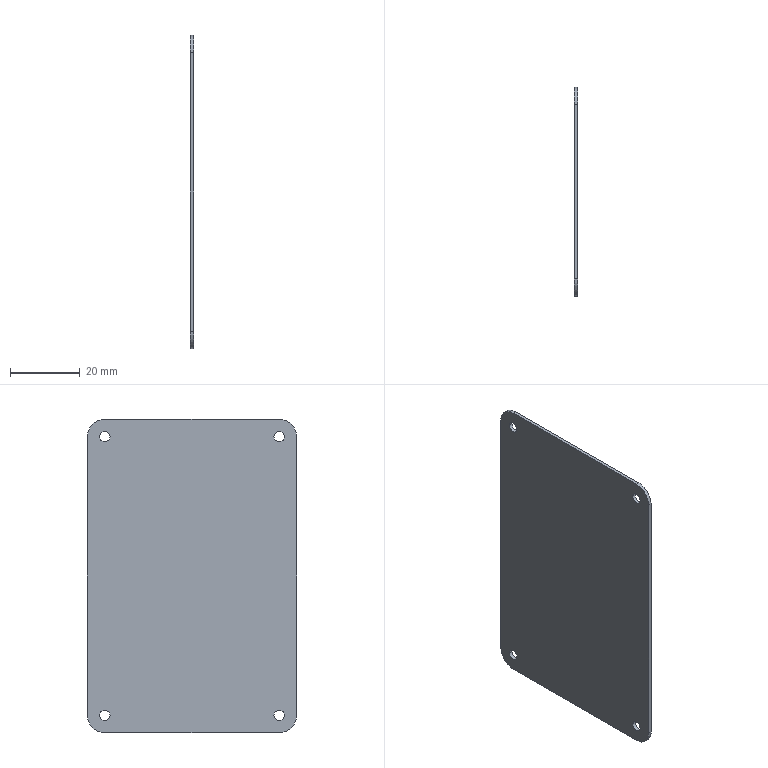Part | Creo | 1 solid | 18 faces | box 1 x 60 x 90 mm | volume 5350 mm3 | cylinder 12 | plane 6 | commonest cylinder face diameters 3 x8 10 x4
STEP:
#1=CARTESIAN_POINT('',(-315.,13.365,-310.635));
#2=VERTEX_POINT('',#1);
#3=CARTESIAN_POINT('',(-315.,-36.635,-310.635));
#4=VERTEX_POINT('',#3);
#5=CARTESIAN_POINT('',(-315.,13.365,-310.635));
#6=DIRECTION('',(0.,-1.,0.));
#7=VECTOR('',#6,50.);
#8=LINE('',#5,#7);
#9=EDGE_CURVE('',#2,#4,#8,.T.);
#10=ORIENTED_EDGE('',*,*,#9,.F.);
#11=CARTESIAN_POINT('',(-315.,18.365,-305.635));
#12=VERTEX_POINT('',#11);
#13=CARTESIAN_POINT('',(-315.,13.365,-305.635));
#14=DIRECTION('',(-1.,0.,0.));
#15=DIRECTION('',(0.,1.,0.));
#16=AXIS2_PLACEMENT_3D('',#13,#14,#15);
#17=CIRCLE('',#16,5.);
#18=EDGE_CURVE('',#12,#2,#17,.T.);
#19=ORIENTED_EDGE('',*,*,#18,.F.);
#20=CARTESIAN_POINT('',(-315.,18.365,-225.635));
#21=VERTEX_POINT('',#20);
#22=CARTESIAN_POINT('',(-315.,18.365,-225.635));
#23=DIRECTION('',(0.,0.,-1.));
#24=VECTOR('',#23,80.);
#25=LINE('',#22,#24);
#26=EDGE_CURVE('',#21,#12,#25,.T.);
#27=ORIENTED_EDGE('',*,*,#26,.F.);
#28=CARTESIAN_POINT('',(-315.,13.365,-220.635));
#29=VERTEX_POINT('',#28);
#30=CARTESIAN_POINT('',(-315.,13.365,-225.635));
#31=DIRECTION('',(-1.,0.,0.));
#32=DIRECTION('',(0.,0.,1.));
#33=AXIS2_PLACEMENT_3D('',#30,#31,#32);
#34=CIRCLE('',#33,5.);
#35=EDGE_CURVE('',#29,#21,#34,.T.);
#36=ORIENTED_EDGE('',*,*,#35,.F.);
#37=CARTESIAN_POINT('',(-315.,-36.635,-220.635));
#38=VERTEX_POINT('',#37);
#39=CARTESIAN_POINT('',(-315.,-36.635,-220.635));
#40=DIRECTION('',(0.,1.,0.));
#41=VECTOR('',#40,50.);
#42=LINE('',#39,#41);
#43=EDGE_CURVE('',#38,#29,#42,.T.);
#44=ORIENTED_EDGE('',*,*,#43,.F.);
#45=CARTESIAN_POINT('',(-315.,-41.635,-225.635));
#46=VERTEX_POINT('',#45);
#47=CARTESIAN_POINT('',(-315.,-36.635,-225.635));
#48=DIRECTION('',(-1.,0.,0.));
#49=DIRECTION('',(0.,-1.,0.));
#50=AXIS2_PLACEMENT_3D('',#47,#48,#49);
#51=CIRCLE('',#50,5.);
#52=EDGE_CURVE('',#46,#38,#51,.T.);
#53=ORIENTED_EDGE('',*,*,#52,.F.);
#54=CARTESIAN_POINT('',(-315.,-41.635,-305.635));
#55=VERTEX_POINT('',#54);
#56=CARTESIAN_POINT('',(-315.,-41.635,-305.635));
#57=DIRECTION('',(0.,0.,1.));
#58=VECTOR('',#57,80.);
#59=LINE('',#56,#58);
#60=EDGE_CURVE('',#55,#46,#59,.T.);
#61=ORIENTED_EDGE('',*,*,#60,.F.);
#62=CARTESIAN_POINT('',(-315.,-36.635,-305.635));
#63=DIRECTION('',(-1.,0.,0.));
#64=DIRECTION('',(0.,0.,-1.));
#65=AXIS2_PLACEMENT_3D('',#62,#63,#64);
#66=CIRCLE('',#65,5.);
#67=EDGE_CURVE('',#4,#55,#66,.T.);
#68=ORIENTED_EDGE('',*,*,#67,.F.);
#69=EDGE_LOOP('',(#10,#19,#27,#36,#44,#53,#61,#68));
#70=FACE_OUTER_BOUND('',#69,.F.);
#71=CARTESIAN_POINT('',(-315.,11.865,-305.635));
#72=VERTEX_POINT('',#71);
#73=CARTESIAN_POINT('',(-315.,14.865,-305.635));
#74=VERTEX_POINT('',#73);
#75=CARTESIAN_POINT('',(-315.,13.365,-305.635));
#76=DIRECTION('',(1.,0.,0.));
#77=DIRECTION('',(0.,-1.,0.));
#78=AXIS2_PLACEMENT_3D('',#75,#76,#77);
#79=CIRCLE('',#78,1.5);
#80=EDGE_CURVE('',#72,#74,#79,.T.);
#81=ORIENTED_EDGE('',*,*,#80,.F.);
#82=CARTESIAN_POINT('',(-315.,13.365,-305.635));
#83=DIRECTION('',(1.,0.,0.));
#84=DIRECTION('',(0.,1.,0.));
#85=AXIS2_PLACEMENT_3D('',#82,#83,#84);
#86=CIRCLE('',#85,1.5);
#87=EDGE_CURVE('',#74,#72,#86,.T.);
#88=ORIENTED_EDGE('',*,*,#87,.F.);
#89=EDGE_LOOP('',(#81,#88));
#90=FACE_BOUND('',#89,.F.);
#91=CARTESIAN_POINT('',(-315.,11.865,-225.635));
#92=VERTEX_POINT('',#91);
#93=CARTESIAN_POINT('',(-315.,14.865,-225.635));
#94=VERTEX_POINT('',#93);
#95=CARTESIAN_POINT('',(-315.,13.365,-225.635));
#96=DIRECTION('',(1.,0.,0.));
#97=DIRECTION('',(0.,-1.,0.));
#98=AXIS2_PLACEMENT_3D('',#95,#96,#97);
#99=CIRCLE('',#98,1.5);
#100=EDGE_CURVE('',#92,#94,#99,.T.);
#101=ORIENTED_EDGE('',*,*,#100,.F.);
#102=CARTESIAN_POINT('',(-315.,13.365,-225.635));
#103=DIRECTION('',(1.,0.,0.));
#104=DIRECTION('',(0.,1.,0.));
#105=AXIS2_PLACEMENT_3D('',#102,#103,#104);
#106=CIRCLE('',#105,1.5);
#107=EDGE_CURVE('',#94,#92,#106,.T.);
#108=ORIENTED_EDGE('',*,*,#107,.F.);
#109=EDGE_LOOP('',(#101,#108));
#110=FACE_BOUND('',#109,.F.);
#111=CARTESIAN_POINT('',(-315.,-38.135,-225.635));
#112=VERTEX_POINT('',#111);
#113=CARTESIAN_POINT('',(-315.,-35.135,-225.635));
#114=VERTEX_POINT('',#113);
#115=CARTESIAN_POINT('',(-315.,-36.635,-225.635));
#116=DIRECTION('',(1.,0.,0.));
#117=DIRECTION('',(0.,-1.,0.));
#118=AXIS2_PLACEMENT_3D('',#115,#116,#117);
#119=CIRCLE('',#118,1.5);
#120=EDGE_CURVE('',#112,#114,#119,.T.);
#121=ORIENTED_EDGE('',*,*,#120,.F.);
#122=CARTESIAN_POINT('',(-315.,-36.635,-225.635));
#123=DIRECTION('',(1.,0.,0.));
#124=DIRECTION('',(0.,1.,0.));
#125=AXIS2_PLACEMENT_3D('',#122,#123,#124);
#126=CIRCLE('',#125,1.5);
#127=EDGE_CURVE('',#114,#112,#126,.T.);
#128=ORIENTED_EDGE('',*,*,#127,.F.);
#129=EDGE_LOOP('',(#121,#128));
#130=FACE_BOUND('',#129,.F.);
#131=CARTESIAN_POINT('',(-315.,-38.135,-305.635));
#132=VERTEX_POINT('',#131);
#133=CARTESIAN_POINT('',(-315.,-35.135,-305.635));
#134=VERTEX_POINT('',#133);
#135=CARTESIAN_POINT('',(-315.,-36.635,-305.635));
#136=DIRECTION('',(1.,0.,0.));
#137=DIRECTION('',(0.,-1.,0.));
#138=AXIS2_PLACEMENT_3D('',#135,#136,#137);
#139=CIRCLE('',#138,1.5);
#140=EDGE_CURVE('',#132,#134,#139,.T.);
#141=ORIENTED_EDGE('',*,*,#140,.F.);
#142=CARTESIAN_POINT('',(-315.,-36.635,-305.635));
#143=DIRECTION('',(1.,0.,0.));
#144=DIRECTION('',(0.,1.,0.));
#145=AXIS2_PLACEMENT_3D('',#142,#143,#144);
#146=CIRCLE('',#145,1.5);
#147=EDGE_CURVE('',#134,#132,#146,.T.);
#148=ORIENTED_EDGE('',*,*,#147,.F.);
#149=EDGE_LOOP('',(#141,#148));
#150=FACE_BOUND('',#149,.F.);
#151=CARTESIAN_POINT('',(-315.,-14.635,-262.635));
#152=DIRECTION('',(1.,0.,0.));
#153=DIRECTION('',(0.,1.,0.));
#154=AXIS2_PLACEMENT_3D('',#151,#152,#153);
#155=PLANE('',#154);
#156=ADVANCED_FACE('',(#70,#90,#110,#130,#150),#155,.F.);
#157=CARTESIAN_POINT('',(-314.,13.365,-310.635));
#158=VERTEX_POINT('',#157);
#159=CARTESIAN_POINT('',(-314.,-36.635,-310.635));
#160=VERTEX_POINT('',#159);
#161=CARTESIAN_POINT('',(-314.,13.365,-310.635));
#162=DIRECTION('',(0.,-1.,0.));
#163=VECTOR('',#162,50.);
#164=LINE('',#161,#163);
#165=EDGE_CURVE('',#158,#160,#164,.T.);
#166=ORIENTED_EDGE('',*,*,#165,.F.);
#167=CARTESIAN_POINT('',(-314.,13.365,-310.635));
#168=DIRECTION('',(-1.,0.,0.));
#169=VECTOR('',#168,1.);
#170=LINE('',#167,#169);
#171=EDGE_CURVE('',#158,#2,#170,.T.);
#172=ORIENTED_EDGE('',*,*,#171,.T.);
#173=ORIENTED_EDGE('',*,*,#9,.T.);
#174=CARTESIAN_POINT('',(-315.,-36.635,-310.635));
#175=DIRECTION('',(1.,0.,0.));
#176=VECTOR('',#175,1.);
#177=LINE('',#174,#176);
#178=EDGE_CURVE('',#4,#160,#177,.T.);
#179=ORIENTED_EDGE('',*,*,#178,.T.);
#180=EDGE_LOOP('',(#166,#172,#173,#179));
#181=FACE_OUTER_BOUND('',#180,.F.);
#182=CARTESIAN_POINT('',(-315.,-41.635,-310.635));
#183=DIRECTION('',(0.,0.,-1.));
#184=DIRECTION('',(0.,-1.,0.));
#185=AXIS2_PLACEMENT_3D('',#182,#183,#184);
#186=PLANE('',#185);
#187=ADVANCED_FACE('',(#181),#186,.T.);
#188=CARTESIAN_POINT('',(-314.,18.365,-225.635));
#189=VERTEX_POINT('',#188);
#190=CARTESIAN_POINT('',(-314.,18.365,-305.635));
#191=VERTEX_POINT('',#190);
#192=CARTESIAN_POINT('',(-314.,18.365,-225.635));
#193=DIRECTION('',(0.,0.,-1.));
#194=VECTOR('',#193,80.);
#195=LINE('',#192,#194);
#196=EDGE_CURVE('',#189,#191,#195,.T.);
#197=ORIENTED_EDGE('',*,*,#196,.T.);
#198=CARTESIAN_POINT('',(-314.,13.365,-305.635));
#199=DIRECTION('',(1.,0.,0.));
#200=DIRECTION('',(0.,0.,-1.));
#201=AXIS2_PLACEMENT_3D('',#198,#199,#200);
#202=CIRCLE('',#201,5.);
#203=EDGE_CURVE('',#158,#191,#202,.T.);
#204=ORIENTED_EDGE('',*,*,#203,.F.);
#205=ORIENTED_EDGE('',*,*,#165,.T.);
#206=CARTESIAN_POINT('',(-314.,-41.635,-305.635));
#207=VERTEX_POINT('',#206);
#208=CARTESIAN_POINT('',(-314.,-36.635,-305.635));
#209=DIRECTION('',(1.,0.,0.));
#210=DIRECTION('',(0.,-1.,0.));
#211=AXIS2_PLACEMENT_3D('',#208,#209,#210);
#212=CIRCLE('',#211,5.);
#213=EDGE_CURVE('',#207,#160,#212,.T.);
#214=ORIENTED_EDGE('',*,*,#213,.F.);
#215=CARTESIAN_POINT('',(-314.,-41.635,-225.635));
#216=VERTEX_POINT('',#215);
#217=CARTESIAN_POINT('',(-314.,-41.635,-305.635));
#218=DIRECTION('',(0.,0.,1.));
#219=VECTOR('',#218,80.);
#220=LINE('',#217,#219);
#221=EDGE_CURVE('',#207,#216,#220,.T.);
#222=ORIENTED_EDGE('',*,*,#221,.T.);
#223=CARTESIAN_POINT('',(-314.,-36.635,-220.635));
#224=VERTEX_POINT('',#223);
#225=CARTESIAN_POINT('',(-314.,-36.635,-225.635));
#226=DIRECTION('',(1.,0.,0.));
#227=DIRECTION('',(0.,0.,1.));
#228=AXIS2_PLACEMENT_3D('',#225,#226,#227);
#229=CIRCLE('',#228,5.);
#230=EDGE_CURVE('',#224,#216,#229,.T.);
#231=ORIENTED_EDGE('',*,*,#230,.F.);
#232=CARTESIAN_POINT('',(-314.,13.365,-220.635));
#233=VERTEX_POINT('',#232);
#234=CARTESIAN_POINT('',(-314.,-36.635,-220.635));
#235=DIRECTION('',(0.,1.,0.));
#236=VECTOR('',#235,50.);
#237=LINE('',#234,#236);
#238=EDGE_CURVE('',#224,#233,#237,.T.);
#239=ORIENTED_EDGE('',*,*,#238,.T.);
#240=CARTESIAN_POINT('',(-314.,13.365,-225.635));
#241=DIRECTION('',(1.,0.,0.));
#242=DIRECTION('',(0.,1.,0.));
#243=AXIS2_PLACEMENT_3D('',#240,#241,#242);
#244=CIRCLE('',#243,5.);
#245=EDGE_CURVE('',#189,#233,#244,.T.);
#246=ORIENTED_EDGE('',*,*,#245,.F.);
#247=EDGE_LOOP('',(#197,#204,#205,#214,#222,#231,#239,#246));
#248=FACE_OUTER_BOUND('',#247,.F.);
#249=CARTESIAN_POINT('',(-314.,14.865,-305.635));
#250=VERTEX_POINT('',#249);
#251=CARTESIAN_POINT('',(-314.,11.865,-305.635));
#252=VERTEX_POINT('',#251);
#253=CARTESIAN_POINT('',(-314.,13.365,-305.635));
#254=DIRECTION('',(-1.,0.,0.));
#255=DIRECTION('',(0.,1.,0.));
#256=AXIS2_PLACEMENT_3D('',#253,#254,#255);
#257=CIRCLE('',#256,1.5);
#258=EDGE_CURVE('',#250,#252,#257,.T.);
#259=ORIENTED_EDGE('',*,*,#258,.F.);
#260=CARTESIAN_POINT('',(-314.,13.365,-305.635));
#261=DIRECTION('',(-1.,0.,0.));
#262=DIRECTION('',(0.,-1.,0.));
#263=AXIS2_PLACEMENT_3D('',#260,#261,#262);
#264=CIRCLE('',#263,1.5);
#265=EDGE_CURVE('',#252,#250,#264,.T.);
#266=ORIENTED_EDGE('',*,*,#265,.F.);
#267=EDGE_LOOP('',(#259,#266));
#268=FACE_BOUND('',#267,.F.);
#269=CARTESIAN_POINT('',(-314.,14.865,-225.635));
#270=VERTEX_POINT('',#269);
#271=CARTESIAN_POINT('',(-314.,11.865,-225.635));
#272=VERTEX_POINT('',#271);
#273=CARTESIAN_POINT('',(-314.,13.365,-225.635));
#274=DIRECTION('',(-1.,0.,0.));
#275=DIRECTION('',(0.,1.,0.));
#276=AXIS2_PLACEMENT_3D('',#273,#274,#275);
#277=CIRCLE('',#276,1.5);
#278=EDGE_CURVE('',#270,#272,#277,.T.);
#279=ORIENTED_EDGE('',*,*,#278,.F.);
#280=CARTESIAN_POINT('',(-314.,13.365,-225.635));
#281=DIRECTION('',(-1.,0.,0.));
#282=DIRECTION('',(0.,-1.,0.));
#283=AXIS2_PLACEMENT_3D('',#280,#281,#282);
#284=CIRCLE('',#283,1.5);
#285=EDGE_CURVE('',#272,#270,#284,.T.);
#286=ORIENTED_EDGE('',*,*,#285,.F.);
#287=EDGE_LOOP('',(#279,#286));
#288=FACE_BOUND('',#287,.F.);
#289=CARTESIAN_POINT('',(-314.,-35.135,-225.635));
#290=VERTEX_POINT('',#289);
#291=CARTESIAN_POINT('',(-314.,-38.135,-225.635));
#292=VERTEX_POINT('',#291);
#293=CARTESIAN_POINT('',(-314.,-36.635,-225.635));
#294=DIRECTION('',(-1.,0.,0.));
#295=DIRECTION('',(0.,1.,0.));
#296=AXIS2_PLACEMENT_3D('',#293,#294,#295);
#297=CIRCLE('',#296,1.5);
#298=EDGE_CURVE('',#290,#292,#297,.T.);
#299=ORIENTED_EDGE('',*,*,#298,.F.);
#300=CARTESIAN_POINT('',(-314.,-36.635,-225.635));
#301=DIRECTION('',(-1.,0.,0.));
#302=DIRECTION('',(0.,-1.,0.));
#303=AXIS2_PLACEMENT_3D('',#300,#301,#302);
#304=CIRCLE('',#303,1.5);
#305=EDGE_CURVE('',#292,#290,#304,.T.);
#306=ORIENTED_EDGE('',*,*,#305,.F.);
#307=EDGE_LOOP('',(#299,#306));
#308=FACE_BOUND('',#307,.F.);
#309=CARTESIAN_POINT('',(-314.,-35.135,-305.635));
#310=VERTEX_POINT('',#309);
#311=CARTESIAN_POINT('',(-314.,-38.135,-305.635));
#312=VERTEX_POINT('',#311);
#313=CARTESIAN_POINT('',(-314.,-36.635,-305.635));
#314=DIRECTION('',(-1.,0.,0.));
#315=DIRECTION('',(0.,1.,0.));
#316=AXIS2_PLACEMENT_3D('',#313,#314,#315);
#317=CIRCLE('',#316,1.5);
#318=EDGE_CURVE('',#310,#312,#317,.T.);
#319=ORIENTED_EDGE('',*,*,#318,.F.);
#320=CARTESIAN_POINT('',(-314.,-36.635,-305.635));
#321=DIRECTION('',(-1.,0.,0.));
#322=DIRECTION('',(0.,-1.,0.));
#323=AXIS2_PLACEMENT_3D('',#320,#321,#322);
#324=CIRCLE('',#323,1.5);
#325=EDGE_CURVE('',#312,#310,#324,.T.);
#326=ORIENTED_EDGE('',*,*,#325,.F.);
#327=EDGE_LOOP('',(#319,#326));
#328=FACE_BOUND('',#327,.F.);
#329=CARTESIAN_POINT('',(-314.,-14.635,-262.635));
#330=DIRECTION('',(1.,0.,0.));
#331=DIRECTION('',(0.,1.,0.));
#332=AXIS2_PLACEMENT_3D('',#329,#330,#331);
#333=PLANE('',#332);
#334=ADVANCED_FACE('',(#248,#268,#288,#308,#328),#333,.T.);
#335=ORIENTED_EDGE('',*,*,#26,.T.);
#336=CARTESIAN_POINT('',(-315.,18.365,-305.635));
#337=DIRECTION('',(1.,0.,0.));
#338=VECTOR('',#337,1.);
#339=LINE('',#336,#338);
#340=EDGE_CURVE('',#12,#191,#339,.T.);
#341=ORIENTED_EDGE('',*,*,#340,.T.);
#342=ORIENTED_EDGE('',*,*,#196,.F.);
#343=CARTESIAN_POINT('',(-314.,18.365,-225.635));
#344=DIRECTION('',(-1.,0.,0.));
#345=VECTOR('',#344,1.);
#346=LINE('',#343,#345);
#347=EDGE_CURVE('',#189,#21,#346,.T.);
#348=ORIENTED_EDGE('',*,*,#347,.T.);
#349=EDGE_LOOP('',(#335,#341,#342,#348));
#350=FACE_OUTER_BOUND('',#349,.F.);
#351=CARTESIAN_POINT('',(-315.,18.365,-310.635));
#352=DIRECTION('',(0.,1.,0.));
#353=DIRECTION('',(0.,0.,-1.));
#354=AXIS2_PLACEMENT_3D('',#351,#352,#353);
#355=PLANE('',#354);
#356=ADVANCED_FACE('',(#350),#355,.T.);
#357=ORIENTED_EDGE('',*,*,#340,.F.);
#358=ORIENTED_EDGE('',*,*,#18,.T.);
#359=ORIENTED_EDGE('',*,*,#171,.F.);
#360=ORIENTED_EDGE('',*,*,#203,.T.);
#361=EDGE_LOOP('',(#357,#358,#359,#360));
#362=FACE_OUTER_BOUND('',#361,.F.);
#363=CARTESIAN_POINT('',(-307.887,13.365,-305.635));
#364=DIRECTION('',(-1.,0.,0.));
#365=DIRECTION('',(0.,-1.,0.));
#366=AXIS2_PLACEMENT_3D('',#363,#364,#365);
#367=CYLINDRICAL_SURFACE('',#366,5.);
#368=ADVANCED_FACE('',(#362),#367,.T.);
#369=CARTESIAN_POINT('',(-315.,13.365,-220.635));
#370=DIRECTION('',(1.,0.,0.));
#371=VECTOR('',#370,1.);
#372=LINE('',#369,#371);
#373=EDGE_CURVE('',#29,#233,#372,.T.);
#374=ORIENTED_EDGE('',*,*,#373,.F.);
#375=ORIENTED_EDGE('',*,*,#35,.T.);
#376=ORIENTED_EDGE('',*,*,#347,.F.);
#377=ORIENTED_EDGE('',*,*,#245,.T.);
#378=EDGE_LOOP('',(#374,#375,#376,#377));
#379=FACE_OUTER_BOUND('',#378,.F.);
#380=CARTESIAN_POINT('',(-307.887,13.365,-225.635));
#381=DIRECTION('',(-1.,0.,0.));
#382=DIRECTION('',(0.,0.,-1.));
#383=AXIS2_PLACEMENT_3D('',#380,#381,#382);
#384=CYLINDRICAL_SURFACE('',#383,5.);
#385=ADVANCED_FACE('',(#379),#384,.T.);
#386=ORIENTED_EDGE('',*,*,#43,.T.);
#387=ORIENTED_EDGE('',*,*,#373,.T.);
#388=ORIENTED_EDGE('',*,*,#238,.F.);
#389=CARTESIAN_POINT('',(-314.,-36.635,-220.635));
#390=DIRECTION('',(-1.,0.,0.));
#391=VECTOR('',#390,1.);
#392=LINE('',#389,#391);
#393=EDGE_CURVE('',#224,#38,#392,.T.);
#394=ORIENTED_EDGE('',*,*,#393,.T.);
#395=EDGE_LOOP('',(#386,#387,#388,#394));
#396=FACE_OUTER_BOUND('',#395,.F.);
#397=CARTESIAN_POINT('',(-315.,18.365,-220.635));
#398=DIRECTION('',(0.,0.,1.));
#399=DIRECTION('',(0.,1.,0.));
#400=AXIS2_PLACEMENT_3D('',#397,#398,#399);
#401=PLANE('',#400);
#402=ADVANCED_FACE('',(#396),#401,.T.);
#403=CARTESIAN_POINT('',(-315.,-41.635,-225.635));
#404=DIRECTION('',(1.,0.,0.));
#405=VECTOR('',#404,1.);
#406=LINE('',#403,#405);
#407=EDGE_CURVE('',#46,#216,#406,.T.);
#408=ORIENTED_EDGE('',*,*,#407,.F.);
#409=ORIENTED_EDGE('',*,*,#52,.T.);
#410=ORIENTED_EDGE('',*,*,#393,.F.);
#411=ORIENTED_EDGE('',*,*,#230,.T.);
#412=EDGE_LOOP('',(#408,#409,#410,#411));
#413=FACE_OUTER_BOUND('',#412,.F.);
#414=CARTESIAN_POINT('',(-307.887,-36.635,-225.635));
#415=DIRECTION('',(-1.,0.,0.));
#416=DIRECTION('',(0.,1.,0.));
#417=AXIS2_PLACEMENT_3D('',#414,#415,#416);
#418=CYLINDRICAL_SURFACE('',#417,5.);
#419=ADVANCED_FACE('',(#413),#418,.T.);
#420=ORIENTED_EDGE('',*,*,#60,.T.);
#421=ORIENTED_EDGE('',*,*,#407,.T.);
#422=ORIENTED_EDGE('',*,*,#221,.F.);
#423=CARTESIAN_POINT('',(-314.,-41.635,-305.635));
#424=DIRECTION('',(-1.,0.,0.));
#425=VECTOR('',#424,1.);
#426=LINE('',#423,#425);
#427=EDGE_CURVE('',#207,#55,#426,.T.);
#428=ORIENTED_EDGE('',*,*,#427,.T.);
#429=EDGE_LOOP('',(#420,#421,#422,#428));
#430=FACE_OUTER_BOUND('',#429,.F.);
#431=CARTESIAN_POINT('',(-315.,-41.635,-220.635));
#432=DIRECTION('',(0.,-1.,0.));
#433=DIRECTION('',(0.,0.,1.));
#434=AXIS2_PLACEMENT_3D('',#431,#432,#433);
#435=PLANE('',#434);
#436=ADVANCED_FACE('',(#430),#435,.T.);
#437=ORIENTED_EDGE('',*,*,#178,.F.);
#438=ORIENTED_EDGE('',*,*,#67,.T.);
#439=ORIENTED_EDGE('',*,*,#427,.F.);
#440=ORIENTED_EDGE('',*,*,#213,.T.);
#441=EDGE_LOOP('',(#437,#438,#439,#440));
#442=FACE_OUTER_BOUND('',#441,.F.);
#443=CARTESIAN_POINT('',(-307.887,-36.635,-305.635));
#444=DIRECTION('',(-1.,0.,0.));
#445=DIRECTION('',(0.,0.,1.));
#446=AXIS2_PLACEMENT_3D('',#443,#444,#445);
#447=CYLINDRICAL_SURFACE('',#446,5.);
#448=ADVANCED_FACE('',(#442),#447,.T.);
#449=CARTESIAN_POINT('',(-315.,11.865,-305.635));
#450=DIRECTION('',(1.,0.,0.));
#451=VECTOR('',#450,1.);
#452=LINE('',#449,#451);
#453=EDGE_CURVE('',#72,#252,#452,.T.);
#454=ORIENTED_EDGE('',*,*,#453,.F.);
#455=ORIENTED_EDGE('',*,*,#80,.T.);
#456=CARTESIAN_POINT('',(-315.,14.865,-305.635));
#457=DIRECTION('',(1.,0.,0.));
#458=VECTOR('',#457,1.);
#459=LINE('',#456,#458);
#460=EDGE_CURVE('',#74,#250,#459,.T.);
#461=ORIENTED_EDGE('',*,*,#460,.T.);
#462=ORIENTED_EDGE('',*,*,#258,.T.);
#463=EDGE_LOOP('',(#454,#455,#461,#462));
#464=FACE_OUTER_BOUND('',#463,.F.);
#465=CARTESIAN_POINT('',(-315.,13.365,-305.635));
#466=DIRECTION('',(1.,0.,0.));
#467=DIRECTION('',(0.,1.,0.));
#468=AXIS2_PLACEMENT_3D('',#465,#466,#467);
#469=CYLINDRICAL_SURFACE('',#468,1.5);
#470=ADVANCED_FACE('',(#464),#469,.F.);
#471=ORIENTED_EDGE('',*,*,#460,.F.);
#472=ORIENTED_EDGE('',*,*,#87,.T.);
#473=ORIENTED_EDGE('',*,*,#453,.T.);
#474=ORIENTED_EDGE('',*,*,#265,.T.);
#475=EDGE_LOOP('',(#471,#472,#473,#474));
#476=FACE_OUTER_BOUND('',#475,.F.);
#477=CARTESIAN_POINT('',(-315.,13.365,-305.635));
#478=DIRECTION('',(1.,0.,0.));
#479=DIRECTION('',(0.,1.,0.));
#480=AXIS2_PLACEMENT_3D('',#477,#478,#479);
#481=CYLINDRICAL_SURFACE('',#480,1.5);
#482=ADVANCED_FACE('',(#476),#481,.F.);
#483=CARTESIAN_POINT('',(-315.,11.865,-225.635));
#484=DIRECTION('',(1.,0.,0.));
#485=VECTOR('',#484,1.);
#486=LINE('',#483,#485);
#487=EDGE_CURVE('',#92,#272,#486,.T.);
#488=ORIENTED_EDGE('',*,*,#487,.F.);
#489=ORIENTED_EDGE('',*,*,#100,.T.);
#490=CARTESIAN_POINT('',(-315.,14.865,-225.635));
#491=DIRECTION('',(1.,0.,0.));
#492=VECTOR('',#491,1.);
#493=LINE('',#490,#492);
#494=EDGE_CURVE('',#94,#270,#493,.T.);
#495=ORIENTED_EDGE('',*,*,#494,.T.);
#496=ORIENTED_EDGE('',*,*,#278,.T.);
#497=EDGE_LOOP('',(#488,#489,#495,#496));
#498=FACE_OUTER_BOUND('',#497,.F.);
#499=CARTESIAN_POINT('',(-315.,13.365,-225.635));
#500=DIRECTION('',(1.,0.,0.));
#501=DIRECTION('',(0.,1.,0.));
#502=AXIS2_PLACEMENT_3D('',#499,#500,#501);
#503=CYLINDRICAL_SURFACE('',#502,1.5);
#504=ADVANCED_FACE('',(#498),#503,.F.);
#505=ORIENTED_EDGE('',*,*,#494,.F.);
#506=ORIENTED_EDGE('',*,*,#107,.T.);
#507=ORIENTED_EDGE('',*,*,#487,.T.);
#508=ORIENTED_EDGE('',*,*,#285,.T.);
#509=EDGE_LOOP('',(#505,#506,#507,#508));
#510=FACE_OUTER_BOUND('',#509,.F.);
#511=CARTESIAN_POINT('',(-315.,13.365,-225.635));
#512=DIRECTION('',(1.,0.,0.));
#513=DIRECTION('',(0.,1.,0.));
#514=AXIS2_PLACEMENT_3D('',#511,#512,#513);
#515=CYLINDRICAL_SURFACE('',#514,1.5);
#516=ADVANCED_FACE('',(#510),#515,.F.);
#517=CARTESIAN_POINT('',(-315.,-38.135,-225.635));
#518=DIRECTION('',(1.,0.,0.));
#519=VECTOR('',#518,1.);
#520=LINE('',#517,#519);
#521=EDGE_CURVE('',#112,#292,#520,.T.);
#522=ORIENTED_EDGE('',*,*,#521,.F.);
#523=ORIENTED_EDGE('',*,*,#120,.T.);
#524=CARTESIAN_POINT('',(-315.,-35.135,-225.635));
#525=DIRECTION('',(1.,0.,0.));
#526=VECTOR('',#525,1.);
#527=LINE('',#524,#526);
#528=EDGE_CURVE('',#114,#290,#527,.T.);
#529=ORIENTED_EDGE('',*,*,#528,.T.);
#530=ORIENTED_EDGE('',*,*,#298,.T.);
#531=EDGE_LOOP('',(#522,#523,#529,#530));
#532=FACE_OUTER_BOUND('',#531,.F.);
#533=CARTESIAN_POINT('',(-315.,-36.635,-225.635));
#534=DIRECTION('',(1.,0.,0.));
#535=DIRECTION('',(0.,1.,0.));
#536=AXIS2_PLACEMENT_3D('',#533,#534,#535);
#537=CYLINDRICAL_SURFACE('',#536,1.5);
#538=ADVANCED_FACE('',(#532),#537,.F.);
#539=ORIENTED_EDGE('',*,*,#528,.F.);
#540=ORIENTED_EDGE('',*,*,#127,.T.);
#541=ORIENTED_EDGE('',*,*,#521,.T.);
#542=ORIENTED_EDGE('',*,*,#305,.T.);
#543=EDGE_LOOP('',(#539,#540,#541,#542));
#544=FACE_OUTER_BOUND('',#543,.F.);
#545=CARTESIAN_POINT('',(-315.,-36.635,-225.635));
#546=DIRECTION('',(1.,0.,0.));
#547=DIRECTION('',(0.,1.,0.));
#548=AXIS2_PLACEMENT_3D('',#545,#546,#547);
#549=CYLINDRICAL_SURFACE('',#548,1.5);
#550=ADVANCED_FACE('',(#544),#549,.F.);
#551=CARTESIAN_POINT('',(-315.,-38.135,-305.635));
#552=DIRECTION('',(1.,0.,0.));
#553=VECTOR('',#552,1.);
#554=LINE('',#551,#553);
#555=EDGE_CURVE('',#132,#312,#554,.T.);
#556=ORIENTED_EDGE('',*,*,#555,.F.);
#557=ORIENTED_EDGE('',*,*,#140,.T.);
#558=CARTESIAN_POINT('',(-315.,-35.135,-305.635));
#559=DIRECTION('',(1.,0.,0.));
#560=VECTOR('',#559,1.);
#561=LINE('',#558,#560);
#562=EDGE_CURVE('',#134,#310,#561,.T.);
#563=ORIENTED_EDGE('',*,*,#562,.T.);
#564=ORIENTED_EDGE('',*,*,#318,.T.);
#565=EDGE_LOOP('',(#556,#557,#563,#564));
#566=FACE_OUTER_BOUND('',#565,.F.);
#567=CARTESIAN_POINT('',(-315.,-36.635,-305.635));
#568=DIRECTION('',(1.,0.,0.));
#569=DIRECTION('',(0.,1.,0.));
#570=AXIS2_PLACEMENT_3D('',#567,#568,#569);
#571=CYLINDRICAL_SURFACE('',#570,1.5);
#572=ADVANCED_FACE('',(#566),#571,.F.);
#573=ORIENTED_EDGE('',*,*,#562,.F.);
#574=ORIENTED_EDGE('',*,*,#147,.T.);
#575=ORIENTED_EDGE('',*,*,#555,.T.);
#576=ORIENTED_EDGE('',*,*,#325,.T.);
#577=EDGE_LOOP('',(#573,#574,#575,#576));
#578=FACE_OUTER_BOUND('',#577,.F.);
#579=CARTESIAN_POINT('',(-315.,-36.635,-305.635));
#580=DIRECTION('',(1.,0.,0.));
#581=DIRECTION('',(0.,1.,0.));
#582=AXIS2_PLACEMENT_3D('',#579,#580,#581);
#583=CYLINDRICAL_SURFACE('',#582,1.5);
#584=ADVANCED_FACE('',(#578),#583,.F.);
#585=CLOSED_SHELL('',(#156,#187,#334,#356,#368,#385,#402,#419,#436,#448,#470,#482,#504,#516,#538,#550,#572,#584));
#586=MANIFOLD_SOLID_BREP('',#585);
#587=(LENGTH_UNIT()NAMED_UNIT(*)SI_UNIT(.MILLI.,.METRE.));
#588=UNCERTAINTY_MEASURE_WITH_UNIT(LENGTH_MEASURE(0.01082),#587,'','');
#589=(NAMED_UNIT(*)PLANE_ANGLE_UNIT()SI_UNIT($,.RADIAN.));
#590=PLANE_ANGLE_MEASURE_WITH_UNIT(PLANE_ANGLE_MEASURE(0.01745),#589);
#591=(CONVERSION_BASED_UNIT('DEGREE',#590)NAMED_UNIT(*)PLANE_ANGLE_UNIT());
#592=(NAMED_UNIT(*)SI_UNIT($,.STERADIAN.)SOLID_ANGLE_UNIT());
#593=(GEOMETRIC_REPRESENTATION_CONTEXT(3)GLOBAL_UNCERTAINTY_ASSIGNED_CONTEXT((#588))GLOBAL_UNIT_ASSIGNED_CONTEXT((#587,#591,#592))REPRESENTATION_CONTEXT('',''));
#594=ADVANCED_BREP_SHAPE_REPRESENTATION('',(#586),#593);